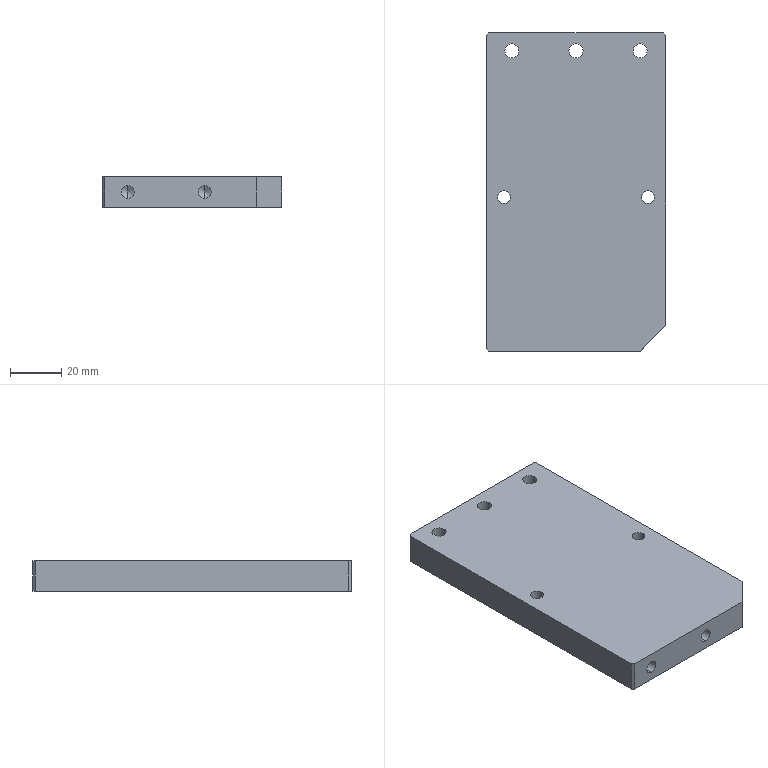Part | STEP file | support plate 29 | 1 solid | 37 faces | box 70 x 124 x 12 mm | volume 100628 mm3 | cylinder 20 | plane 13 | cone 4 | commonest cylinder face diameters 5 x8 5.5 x6 10 x6